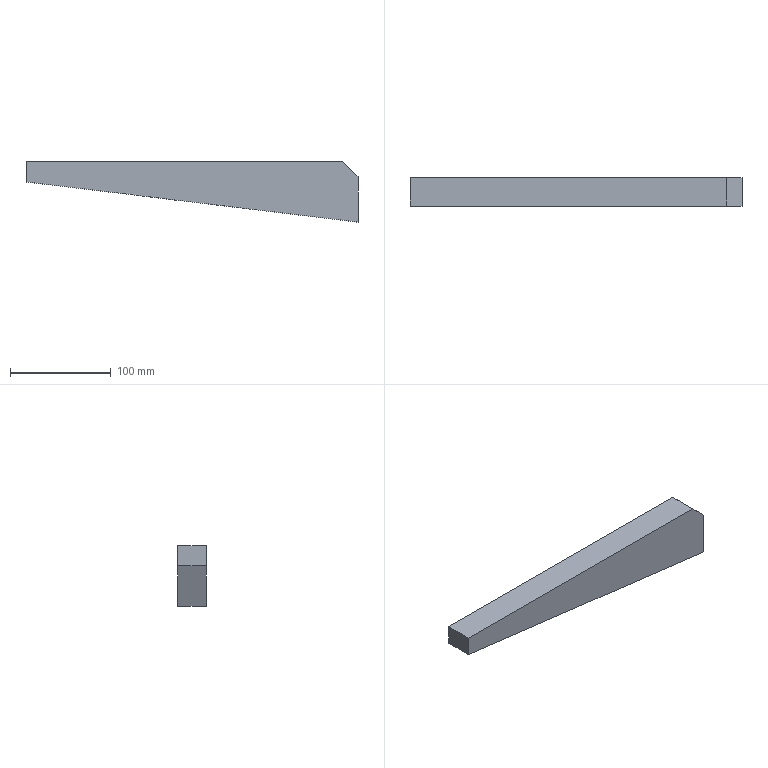Part | SolidWorks | features Extrusion 1 | 1 solid | 7 faces | box 330 x 28 x 60 mm | volume 366450 mm3 | plane 7
STEP:
#1=CARTESIAN_POINT('',(2750.873,0.,-1624.163));
#2=VERTEX_POINT('',#1);
#3=CARTESIAN_POINT('',(2750.873,0.,-1604.163));
#4=VERTEX_POINT('',#3);
#5=CARTESIAN_POINT('',(2750.873,0.,-1624.163));
#6=DIRECTION('',(0.,0.,1.));
#7=VECTOR('',#6,1000.);
#8=LINE('',#5,#7);
#9=EDGE_CURVE('',#2,#4,#8,.T.);
#10=ORIENTED_EDGE('',*,*,#9,.T.);
#11=CARTESIAN_POINT('',(2750.873,28.,-1604.163));
#12=VERTEX_POINT('',#11);
#13=CARTESIAN_POINT('',(2750.873,28.,-1604.163));
#14=DIRECTION('',(0.,-1.,0.));
#15=VECTOR('',#14,1000.);
#16=LINE('',#13,#15);
#17=EDGE_CURVE('',#12,#4,#16,.T.);
#18=ORIENTED_EDGE('',*,*,#17,.F.);
#19=CARTESIAN_POINT('',(2750.873,28.,-1624.163));
#20=VERTEX_POINT('',#19);
#21=CARTESIAN_POINT('',(2750.873,28.,-1624.163));
#22=DIRECTION('',(0.,0.,1.));
#23=VECTOR('',#22,1000.);
#24=LINE('',#21,#23);
#25=EDGE_CURVE('',#20,#12,#24,.T.);
#26=ORIENTED_EDGE('',*,*,#25,.F.);
#27=CARTESIAN_POINT('',(2750.873,28.,-1624.163));
#28=DIRECTION('',(0.,-1.,0.));
#29=VECTOR('',#28,1000.);
#30=LINE('',#27,#29);
#31=EDGE_CURVE('',#20,#2,#30,.T.);
#32=ORIENTED_EDGE('',*,*,#31,.T.);
#33=EDGE_LOOP('',(#10,#18,#26,#32));
#34=FACE_OUTER_BOUND('',#33,.T.);
#35=CARTESIAN_POINT('',(2750.873,28.,-1624.163));
#36=DIRECTION('',(1.,0.,0.));
#37=DIRECTION('',(0.,0.,-1.));
#38=AXIS2_PLACEMENT_3D('',#35,#36,#37);
#39=PLANE('',#38);
#40=ADVANCED_FACE('',(#34),#39,.F.);
#41=CARTESIAN_POINT('',(3065.873,0.,-1604.163));
#42=VERTEX_POINT('',#41);
#43=CARTESIAN_POINT('',(2750.873,0.,-1604.163));
#44=DIRECTION('',(1.,0.,0.));
#45=VECTOR('',#44,1000.);
#46=LINE('',#43,#45);
#47=EDGE_CURVE('',#4,#42,#46,.T.);
#48=ORIENTED_EDGE('',*,*,#47,.T.);
#49=CARTESIAN_POINT('',(3065.873,28.,-1604.163));
#50=VERTEX_POINT('',#49);
#51=CARTESIAN_POINT('',(3065.873,28.,-1604.163));
#52=DIRECTION('',(0.,-1.,0.));
#53=VECTOR('',#52,1000.);
#54=LINE('',#51,#53);
#55=EDGE_CURVE('',#50,#42,#54,.T.);
#56=ORIENTED_EDGE('',*,*,#55,.F.);
#57=CARTESIAN_POINT('',(2750.873,28.,-1604.163));
#58=DIRECTION('',(1.,0.,0.));
#59=VECTOR('',#58,1000.);
#60=LINE('',#57,#59);
#61=EDGE_CURVE('',#12,#50,#60,.T.);
#62=ORIENTED_EDGE('',*,*,#61,.F.);
#63=ORIENTED_EDGE('',*,*,#17,.T.);
#64=EDGE_LOOP('',(#48,#56,#62,#63));
#65=FACE_OUTER_BOUND('',#64,.T.);
#66=CARTESIAN_POINT('',(2750.873,28.,-1604.163));
#67=DIRECTION('',(0.,0.,-1.));
#68=DIRECTION('',(-1.,0.,0.));
#69=AXIS2_PLACEMENT_3D('',#66,#67,#68);
#70=PLANE('',#69);
#71=ADVANCED_FACE('',(#65),#70,.F.);
#72=CARTESIAN_POINT('',(3080.873,0.,-1619.163));
#73=VERTEX_POINT('',#72);
#74=CARTESIAN_POINT('',(3065.873,0.,-1604.163));
#75=DIRECTION('',(0.7071,0.,-0.7071));
#76=VECTOR('',#75,1000.);
#77=LINE('',#74,#76);
#78=EDGE_CURVE('',#42,#73,#77,.T.);
#79=ORIENTED_EDGE('',*,*,#78,.T.);
#80=CARTESIAN_POINT('',(3080.873,28.,-1619.163));
#81=VERTEX_POINT('',#80);
#82=CARTESIAN_POINT('',(3080.873,28.,-1619.163));
#83=DIRECTION('',(0.,-1.,0.));
#84=VECTOR('',#83,1000.);
#85=LINE('',#82,#84);
#86=EDGE_CURVE('',#81,#73,#85,.T.);
#87=ORIENTED_EDGE('',*,*,#86,.F.);
#88=CARTESIAN_POINT('',(3065.873,28.,-1604.163));
#89=DIRECTION('',(0.7071,0.,-0.7071));
#90=VECTOR('',#89,1000.);
#91=LINE('',#88,#90);
#92=EDGE_CURVE('',#50,#81,#91,.T.);
#93=ORIENTED_EDGE('',*,*,#92,.F.);
#94=ORIENTED_EDGE('',*,*,#55,.T.);
#95=EDGE_LOOP('',(#79,#87,#93,#94));
#96=FACE_OUTER_BOUND('',#95,.T.);
#97=CARTESIAN_POINT('',(3065.873,28.,-1604.163));
#98=DIRECTION('',(-0.7071,0.,-0.7071));
#99=DIRECTION('',(-0.7071,0.,0.7071));
#100=AXIS2_PLACEMENT_3D('',#97,#98,#99);
#101=PLANE('',#100);
#102=ADVANCED_FACE('',(#96),#101,.F.);
#103=CARTESIAN_POINT('',(3080.873,0.,-1664.163));
#104=VERTEX_POINT('',#103);
#105=CARTESIAN_POINT('',(3080.873,0.,-1619.163));
#106=DIRECTION('',(0.,0.,-1.));
#107=VECTOR('',#106,1000.);
#108=LINE('',#105,#107);
#109=EDGE_CURVE('',#73,#104,#108,.T.);
#110=ORIENTED_EDGE('',*,*,#109,.T.);
#111=CARTESIAN_POINT('',(3080.873,28.,-1664.163));
#112=VERTEX_POINT('',#111);
#113=CARTESIAN_POINT('',(3080.873,28.,-1664.163));
#114=DIRECTION('',(0.,-1.,0.));
#115=VECTOR('',#114,1000.);
#116=LINE('',#113,#115);
#117=EDGE_CURVE('',#112,#104,#116,.T.);
#118=ORIENTED_EDGE('',*,*,#117,.F.);
#119=CARTESIAN_POINT('',(3080.873,28.,-1619.163));
#120=DIRECTION('',(0.,0.,-1.));
#121=VECTOR('',#120,1000.);
#122=LINE('',#119,#121);
#123=EDGE_CURVE('',#81,#112,#122,.T.);
#124=ORIENTED_EDGE('',*,*,#123,.F.);
#125=ORIENTED_EDGE('',*,*,#86,.T.);
#126=EDGE_LOOP('',(#110,#118,#124,#125));
#127=FACE_OUTER_BOUND('',#126,.T.);
#128=CARTESIAN_POINT('',(3080.873,28.,-1619.163));
#129=DIRECTION('',(-1.,0.,0.));
#130=DIRECTION('',(0.,0.,1.));
#131=AXIS2_PLACEMENT_3D('',#128,#129,#130);
#132=PLANE('',#131);
#133=ADVANCED_FACE('',(#127),#132,.F.);
#134=CARTESIAN_POINT('',(3080.873,0.,-1664.163));
#135=DIRECTION('',(-0.9927,0.,0.1203));
#136=VECTOR('',#135,1000.);
#137=LINE('',#134,#136);
#138=EDGE_CURVE('',#104,#2,#137,.T.);
#139=ORIENTED_EDGE('',*,*,#138,.T.);
#140=ORIENTED_EDGE('',*,*,#31,.F.);
#141=CARTESIAN_POINT('',(3080.873,28.,-1664.163));
#142=DIRECTION('',(-0.9927,0.,0.1203));
#143=VECTOR('',#142,1000.);
#144=LINE('',#141,#143);
#145=EDGE_CURVE('',#112,#20,#144,.T.);
#146=ORIENTED_EDGE('',*,*,#145,.F.);
#147=ORIENTED_EDGE('',*,*,#117,.T.);
#148=EDGE_LOOP('',(#139,#140,#146,#147));
#149=FACE_OUTER_BOUND('',#148,.T.);
#150=CARTESIAN_POINT('',(3080.873,28.,-1664.163));
#151=DIRECTION('',(0.1203,0.,0.9927));
#152=DIRECTION('',(0.9927,0.,-0.1203));
#153=AXIS2_PLACEMENT_3D('',#150,#151,#152);
#154=PLANE('',#153);
#155=ADVANCED_FACE('',(#149),#154,.F.);
#156=ORIENTED_EDGE('',*,*,#25,.T.);
#157=ORIENTED_EDGE('',*,*,#61,.T.);
#158=ORIENTED_EDGE('',*,*,#92,.T.);
#159=ORIENTED_EDGE('',*,*,#123,.T.);
#160=ORIENTED_EDGE('',*,*,#145,.T.);
#161=EDGE_LOOP('',(#156,#157,#158,#159,#160));
#162=FACE_OUTER_BOUND('',#161,.T.);
#163=CARTESIAN_POINT('',(0.,28.,0.));
#164=DIRECTION('',(0.,1.,0.));
#165=DIRECTION('',(0.,0.,1.));
#166=AXIS2_PLACEMENT_3D('',#163,#164,#165);
#167=PLANE('',#166);
#168=ADVANCED_FACE('',(#162),#167,.T.);
#169=ORIENTED_EDGE('',*,*,#9,.F.);
#170=ORIENTED_EDGE('',*,*,#138,.F.);
#171=ORIENTED_EDGE('',*,*,#109,.F.);
#172=ORIENTED_EDGE('',*,*,#78,.F.);
#173=ORIENTED_EDGE('',*,*,#47,.F.);
#174=EDGE_LOOP('',(#169,#170,#171,#172,#173));
#175=FACE_OUTER_BOUND('',#174,.T.);
#176=CARTESIAN_POINT('',(0.,0.,0.));
#177=DIRECTION('',(0.,1.,0.));
#178=DIRECTION('',(0.,0.,1.));
#179=AXIS2_PLACEMENT_3D('',#176,#177,#178);
#180=PLANE('',#179);
#181=ADVANCED_FACE('',(#175),#180,.F.);
#182=CLOSED_SHELL('',(#40,#71,#102,#133,#155,#168,#181));
#183=MANIFOLD_SOLID_BREP('',#182);
#184=CARTESIAN_POINT('',(0.,0.,0.));
#185=DIRECTION('',(0.,0.,1.));
#186=DIRECTION('',(1.,0.,0.));
#187=AXIS2_PLACEMENT_3D('',#184,#185,#186);
#188=(LENGTH_UNIT()NAMED_UNIT(*)SI_UNIT(.MILLI.,.METRE.));
#189=UNCERTAINTY_MEASURE_WITH_UNIT(LENGTH_MEASURE(0.00001),#188,'','');
#190=(NAMED_UNIT(*)PLANE_ANGLE_UNIT()SI_UNIT($,.RADIAN.));
#191=(NAMED_UNIT(*)SI_UNIT($,.STERADIAN.)SOLID_ANGLE_UNIT());
#192=(GEOMETRIC_REPRESENTATION_CONTEXT(3)GLOBAL_UNCERTAINTY_ASSIGNED_CONTEXT((#189))GLOBAL_UNIT_ASSIGNED_CONTEXT((#188,#190,#191))REPRESENTATION_CONTEXT('',''));
#193=ADVANCED_BREP_SHAPE_REPRESENTATION('',(#183,#187),#192);